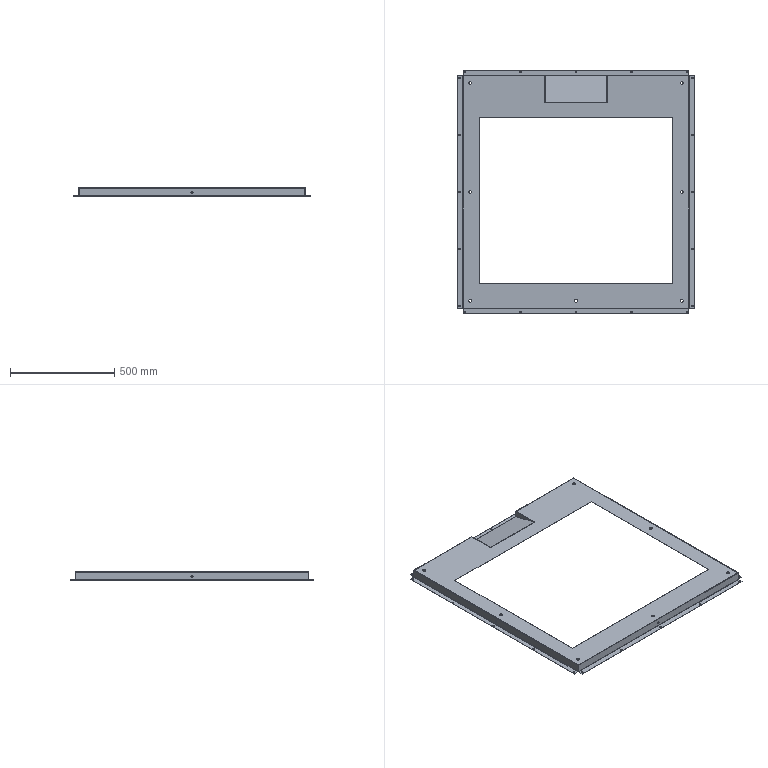Part | 2 solids | 214 faces | box 1139 x 1169 x 40 mm | volume 751530 mm3 | plane 110 | cylinder 92 | spline 12 | commonest cylinder face diameters 7 x50 14 x14 0.4 x11 2.4 x11 10 x6